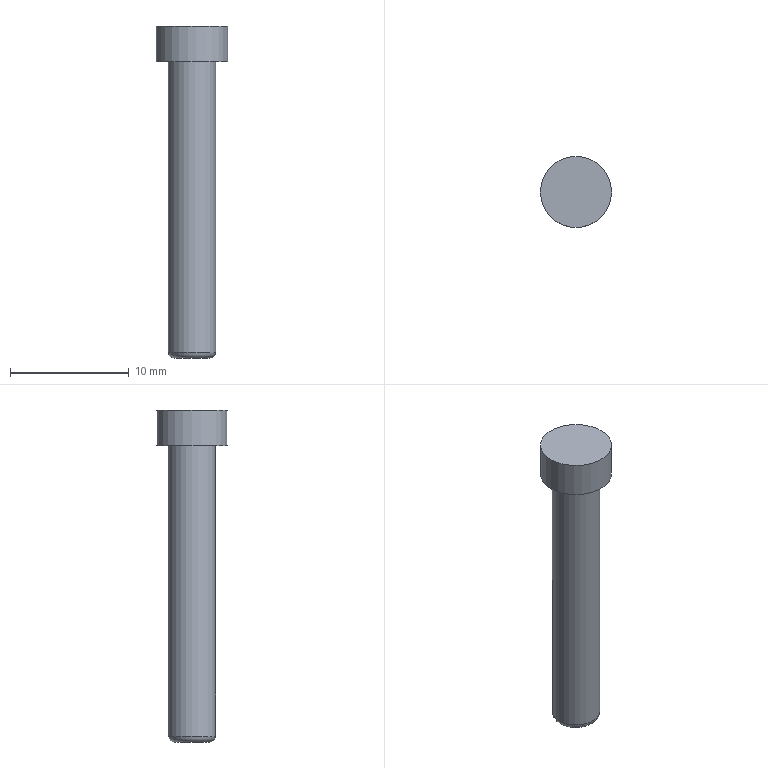Part | NX | features solid 2 | 1 solid | 6 faces | box 6 x 6 x 28 mm | volume 398.346 mm3 | plane 3 | cylinder 2 | torus 1 | commonest cylinder face diameters 4 x1 6 x1
STEP:
#1=CARTESIAN_POINT('',(765.378,-23.978,-10.5));
#2=VERTEX_POINT('',#1);
#3=CARTESIAN_POINT('',(766.878,-23.978,-10.5));
#4=DIRECTION('',(0.,0.,-1.));
#5=DIRECTION('',(-1.,0.,0.));
#6=AXIS2_PLACEMENT_3D('',#3,#4,#5);
#7=CIRCLE('',#6,1.5);
#8=EDGE_CURVE('',#2,#2,#7,.T.);
#9=ORIENTED_EDGE('',*,*,#8,.T.);
#10=EDGE_LOOP('',(#9));
#11=FACE_BOUND('',#10,.T.);
#12=CARTESIAN_POINT('',(766.878,-23.978,-10.5));
#13=DIRECTION('',(0.,0.,-1.));
#14=DIRECTION('',(-1.,0.,0.));
#15=AXIS2_PLACEMENT_3D('',#12,#13,#14);
#16=PLANE('',#15);
#17=ADVANCED_FACE('',(#11),#16,.T.);
#18=CARTESIAN_POINT('',(764.878,-23.978,14.5));
#19=VERTEX_POINT('',#18);
#20=CARTESIAN_POINT('',(766.878,-23.978,14.5));
#21=DIRECTION('',(0.,0.,-1.));
#22=DIRECTION('',(-1.,0.,0.));
#23=AXIS2_PLACEMENT_3D('',#20,#21,#22);
#24=CIRCLE('',#23,2.);
#25=EDGE_CURVE('',#19,#19,#24,.F.);
#26=ORIENTED_EDGE('',*,*,#25,.F.);
#27=EDGE_LOOP('',(#26));
#28=FACE_BOUND('',#27,.T.);
#29=CARTESIAN_POINT('',(764.878,-23.978,-10.));
#30=VERTEX_POINT('',#29);
#31=CARTESIAN_POINT('',(766.878,-23.978,-10.));
#32=DIRECTION('',(0.,0.,-1.));
#33=DIRECTION('',(-1.,0.,0.));
#34=AXIS2_PLACEMENT_3D('',#31,#32,#33);
#35=CIRCLE('',#34,2.);
#36=EDGE_CURVE('',#30,#30,#35,.F.);
#37=ORIENTED_EDGE('',*,*,#36,.T.);
#38=EDGE_LOOP('',(#37));
#39=FACE_BOUND('',#38,.T.);
#40=CARTESIAN_POINT('',(766.878,-23.978,32.5));
#41=DIRECTION('',(0.,0.,-1.));
#42=DIRECTION('',(1.,0.,0.));
#43=AXIS2_PLACEMENT_3D('',#40,#41,#42);
#44=CYLINDRICAL_SURFACE('',#43,2.);
#45=ADVANCED_FACE('',(#28,#39),#44,.T.);
#46=ORIENTED_EDGE('',*,*,#8,.F.);
#47=EDGE_LOOP('',(#46));
#48=FACE_BOUND('',#47,.T.);
#49=ORIENTED_EDGE('',*,*,#36,.F.);
#50=EDGE_LOOP('',(#49));
#51=FACE_BOUND('',#50,.T.);
#52=CARTESIAN_POINT('',(766.878,-23.978,-10.));
#53=DIRECTION('',(0.,0.,-1.));
#54=DIRECTION('',(-1.,0.,0.));
#55=AXIS2_PLACEMENT_3D('',#52,#53,#54);
#56=TOROIDAL_SURFACE('',#55,1.5,0.5);
#57=ADVANCED_FACE('',(#48,#51),#56,.T.);
#58=ORIENTED_EDGE('',*,*,#25,.T.);
#59=EDGE_LOOP('',(#58));
#60=FACE_BOUND('',#59,.T.);
#61=CARTESIAN_POINT('',(769.878,-23.978,14.5));
#62=VERTEX_POINT('',#61);
#63=CARTESIAN_POINT('',(766.878,-23.978,14.5));
#64=DIRECTION('',(0.,0.,1.));
#65=DIRECTION('',(1.,0.,0.));
#66=AXIS2_PLACEMENT_3D('',#63,#64,#65);
#67=CIRCLE('',#66,3.);
#68=EDGE_CURVE('',#62,#62,#67,.T.);
#69=ORIENTED_EDGE('',*,*,#68,.F.);
#70=EDGE_LOOP('',(#69));
#71=FACE_BOUND('',#70,.T.);
#72=CARTESIAN_POINT('',(766.878,-23.978,14.5));
#73=DIRECTION('',(0.,0.,-1.));
#74=DIRECTION('',(-1.,0.,0.));
#75=AXIS2_PLACEMENT_3D('',#72,#73,#74);
#76=PLANE('',#75);
#77=ADVANCED_FACE('',(#60,#71),#76,.T.);
#78=ORIENTED_EDGE('',*,*,#68,.T.);
#79=EDGE_LOOP('',(#78));
#80=FACE_BOUND('',#79,.T.);
#81=CARTESIAN_POINT('',(769.878,-23.978,17.5));
#82=VERTEX_POINT('',#81);
#83=CARTESIAN_POINT('',(766.878,-23.978,17.5));
#84=DIRECTION('',(0.,0.,-1.));
#85=DIRECTION('',(1.,0.,0.));
#86=AXIS2_PLACEMENT_3D('',#83,#84,#85);
#87=CIRCLE('',#86,3.);
#88=EDGE_CURVE('',#82,#82,#87,.T.);
#89=ORIENTED_EDGE('',*,*,#88,.T.);
#90=EDGE_LOOP('',(#89));
#91=FACE_BOUND('',#90,.T.);
#92=CARTESIAN_POINT('',(766.878,-23.978,17.5));
#93=DIRECTION('',(0.,0.,-1.));
#94=DIRECTION('',(1.,0.,0.));
#95=AXIS2_PLACEMENT_3D('',#92,#93,#94);
#96=CYLINDRICAL_SURFACE('',#95,3.);
#97=ADVANCED_FACE('',(#80,#91),#96,.T.);
#98=ORIENTED_EDGE('',*,*,#88,.F.);
#99=EDGE_LOOP('',(#98));
#100=FACE_BOUND('',#99,.T.);
#101=CARTESIAN_POINT('',(766.878,-23.978,17.5));
#102=DIRECTION('',(0.,0.,1.));
#103=DIRECTION('',(1.,0.,0.));
#104=AXIS2_PLACEMENT_3D('',#101,#102,#103);
#105=PLANE('',#104);
#106=ADVANCED_FACE('',(#100),#105,.T.);
#107=CLOSED_SHELL('',(#17,#45,#57,#77,#97,#106));
#108=MANIFOLD_SOLID_BREP('',#107);
#109=(LENGTH_UNIT()NAMED_UNIT(*)SI_UNIT(.MILLI.,.METRE.));
#110=UNCERTAINTY_MEASURE_WITH_UNIT(LENGTH_MEASURE(0.00001),#109,'','');
#111=(NAMED_UNIT(*)PLANE_ANGLE_UNIT()SI_UNIT($,.RADIAN.));
#112=(NAMED_UNIT(*)SI_UNIT($,.STERADIAN.)SOLID_ANGLE_UNIT());
#113=(GEOMETRIC_REPRESENTATION_CONTEXT(3)GLOBAL_UNCERTAINTY_ASSIGNED_CONTEXT((#110))GLOBAL_UNIT_ASSIGNED_CONTEXT((#109,#111,#112))REPRESENTATION_CONTEXT('',''));
#114=ADVANCED_BREP_SHAPE_REPRESENTATION('',(#108),#113);